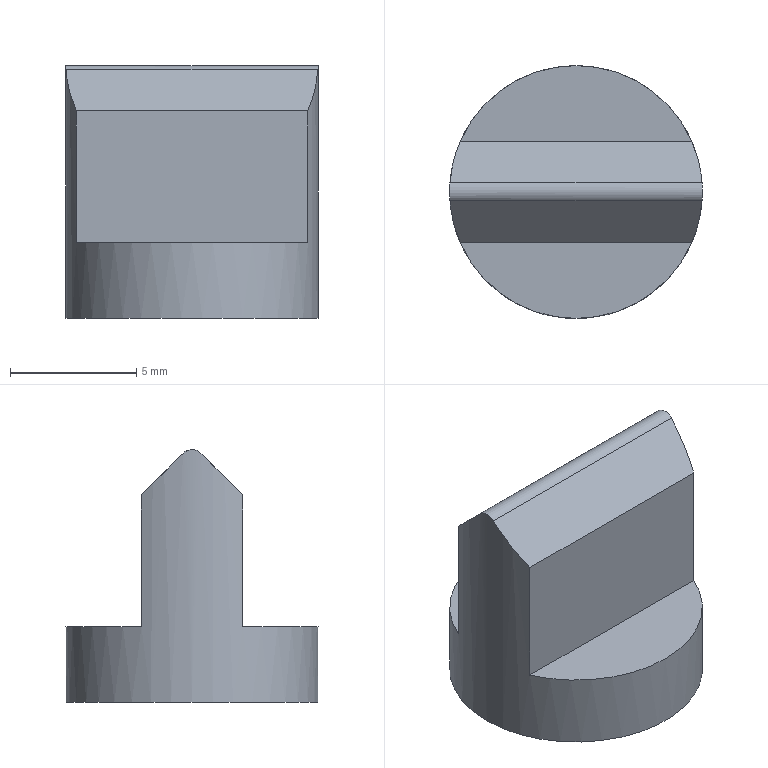Part | STEP file | lll_id294_x_t | 1 solid | 9 faces | box 10 x 10 x 10 mm | volume 477.247 mm3 | plane 7 | cylinder 2 | commonest cylinder face diameters 1 x1 10 x1
STEP:
#1=CARTESIAN_POINT('',(5.,106.,-20.));
#2=VERTEX_POINT('',#1);
#3=CARTESIAN_POINT('',(0.,106.,-20.));
#4=DIRECTION('',(0.,0.,1.));
#5=DIRECTION('',(1.,0.,0.));
#6=AXIS2_PLACEMENT_3D('',#3,#4,#5);
#7=CIRCLE('',#6,5.);
#8=EDGE_CURVE('',#2,#2,#7,.T.);
#9=ORIENTED_EDGE('',*,*,#8,.F.);
#10=EDGE_LOOP('',(#9));
#11=FACE_OUTER_BOUND('',#10,.T.);
#12=CARTESIAN_POINT('',(48.194,357.,-20.));
#13=DIRECTION('',(0.,0.,-1.));
#14=DIRECTION('',(1.,0.,0.));
#15=AXIS2_PLACEMENT_3D('',#12,#13,#14);
#16=PLANE('',#15);
#17=ADVANCED_FACE('',(#11),#16,.T.);
#18=CARTESIAN_POINT('',(-4.583,104.,-17.));
#19=VERTEX_POINT('',#18);
#20=CARTESIAN_POINT('',(-4.583,104.,-11.793));
#21=VERTEX_POINT('',#20);
#22=CARTESIAN_POINT('',(-4.583,104.,-22.));
#23=DIRECTION('',(0.,0.,1.));
#24=VECTOR('',#23,1.);
#25=LINE('',#22,#24);
#26=EDGE_CURVE('',#19,#21,#25,.T.);
#27=ORIENTED_EDGE('',*,*,#26,.F.);
#28=CARTESIAN_POINT('',(4.583,104.,-17.));
#29=VERTEX_POINT('',#28);
#30=CARTESIAN_POINT('',(13.,104.,-17.));
#31=DIRECTION('',(-1.,0.,0.));
#32=VECTOR('',#31,1.);
#33=LINE('',#30,#32);
#34=EDGE_CURVE('',#29,#19,#33,.T.);
#35=ORIENTED_EDGE('',*,*,#34,.F.);
#36=CARTESIAN_POINT('',(4.583,104.,-11.793));
#37=VERTEX_POINT('',#36);
#38=CARTESIAN_POINT('',(4.583,104.,-22.));
#39=DIRECTION('',(0.,0.,-1.));
#40=VECTOR('',#39,1.);
#41=LINE('',#38,#40);
#42=EDGE_CURVE('',#37,#29,#41,.T.);
#43=ORIENTED_EDGE('',*,*,#42,.F.);
#44=CARTESIAN_POINT('',(13.,104.,-11.793));
#45=DIRECTION('',(-1.,0.,0.));
#46=VECTOR('',#45,1.);
#47=LINE('',#44,#46);
#48=EDGE_CURVE('',#37,#21,#47,.T.);
#49=ORIENTED_EDGE('',*,*,#48,.T.);
#50=EDGE_LOOP('',(#27,#35,#43,#49));
#51=FACE_OUTER_BOUND('',#50,.T.);
#52=CARTESIAN_POINT('',(13.,104.,-11.5));
#53=DIRECTION('',(0.,1.,0.));
#54=DIRECTION('',(0.,0.,-1.));
#55=AXIS2_PLACEMENT_3D('',#52,#53,#54);
#56=PLANE('',#55);
#57=ADVANCED_FACE('',(#51),#56,.F.);
#58=CARTESIAN_POINT('',(-4.583,108.,-17.));
#59=VERTEX_POINT('',#58);
#60=CARTESIAN_POINT('',(4.583,108.,-17.));
#61=VERTEX_POINT('',#60);
#62=CARTESIAN_POINT('',(0.,106.,-17.));
#63=DIRECTION('',(0.,0.,-1.));
#64=DIRECTION('',(1.,0.,0.));
#65=AXIS2_PLACEMENT_3D('',#62,#63,#64);
#66=CIRCLE('',#65,5.);
#67=EDGE_CURVE('',#59,#61,#66,.T.);
#68=ORIENTED_EDGE('',*,*,#67,.F.);
#69=CARTESIAN_POINT('',(13.,108.,-17.));
#70=DIRECTION('',(-1.,0.,0.));
#71=VECTOR('',#70,1.);
#72=LINE('',#69,#71);
#73=EDGE_CURVE('',#61,#59,#72,.T.);
#74=ORIENTED_EDGE('',*,*,#73,.F.);
#75=EDGE_LOOP('',(#68,#74));
#76=FACE_OUTER_BOUND('',#75,.T.);
#77=CARTESIAN_POINT('',(13.,111.,-17.));
#78=DIRECTION('',(0.,0.,-1.));
#79=DIRECTION('',(0.,-1.,0.));
#80=AXIS2_PLACEMENT_3D('',#77,#78,#79);
#81=PLANE('',#80);
#82=ADVANCED_FACE('',(#76),#81,.F.);
#83=CARTESIAN_POINT('',(4.583,108.,-11.793));
#84=VERTEX_POINT('',#83);
#85=CARTESIAN_POINT('',(4.583,108.,-22.));
#86=DIRECTION('',(0.,0.,1.));
#87=VECTOR('',#86,1.);
#88=LINE('',#85,#87);
#89=EDGE_CURVE('',#61,#84,#88,.T.);
#90=ORIENTED_EDGE('',*,*,#89,.F.);
#91=ORIENTED_EDGE('',*,*,#73,.T.);
#92=CARTESIAN_POINT('',(-4.583,108.,-11.793));
#93=VERTEX_POINT('',#92);
#94=CARTESIAN_POINT('',(-4.583,108.,-22.));
#95=DIRECTION('',(0.,0.,-1.));
#96=VECTOR('',#95,1.);
#97=LINE('',#94,#96);
#98=EDGE_CURVE('',#93,#59,#97,.T.);
#99=ORIENTED_EDGE('',*,*,#98,.F.);
#100=CARTESIAN_POINT('',(13.,108.,-11.793));
#101=DIRECTION('',(-1.,0.,0.));
#102=VECTOR('',#101,1.);
#103=LINE('',#100,#102);
#104=EDGE_CURVE('',#84,#93,#103,.T.);
#105=ORIENTED_EDGE('',*,*,#104,.F.);
#106=EDGE_LOOP('',(#90,#91,#99,#105));
#107=FACE_OUTER_BOUND('',#106,.T.);
#108=CARTESIAN_POINT('',(13.,108.,-17.));
#109=DIRECTION('',(0.,-1.,0.));
#110=DIRECTION('',(0.,0.,1.));
#111=AXIS2_PLACEMENT_3D('',#108,#109,#110);
#112=PLANE('',#111);
#113=ADVANCED_FACE('',(#107),#112,.F.);
#114=CARTESIAN_POINT('',(-4.987,106.354,-10.146));
#115=VERTEX_POINT('',#114);
#116=CARTESIAN_POINT('',(0.,106.,-9.793));
#117=DIRECTION('',(0.,-0.7071,-0.7071));
#118=DIRECTION('',(0.,-0.7071,0.7071));
#119=AXIS2_PLACEMENT_3D('',#116,#117,#118);
#120=ELLIPSE('',#119,7.071,5.);
#121=EDGE_CURVE('',#115,#93,#120,.T.);
#122=ORIENTED_EDGE('',*,*,#121,.F.);
#123=CARTESIAN_POINT('',(4.987,106.354,-10.146));
#124=VERTEX_POINT('',#123);
#125=CARTESIAN_POINT('',(13.,106.354,-10.146));
#126=DIRECTION('',(-1.,0.,0.));
#127=VECTOR('',#126,1.);
#128=LINE('',#125,#127);
#129=EDGE_CURVE('',#124,#115,#128,.T.);
#130=ORIENTED_EDGE('',*,*,#129,.F.);
#131=CARTESIAN_POINT('',(0.,106.,-9.793));
#132=DIRECTION('',(0.,-0.7071,-0.7071));
#133=DIRECTION('',(0.,-0.7071,0.7071));
#134=AXIS2_PLACEMENT_3D('',#131,#132,#133);
#135=ELLIPSE('',#134,7.071,5.);
#136=EDGE_CURVE('',#84,#124,#135,.T.);
#137=ORIENTED_EDGE('',*,*,#136,.F.);
#138=ORIENTED_EDGE('',*,*,#104,.T.);
#139=EDGE_LOOP('',(#122,#130,#137,#138));
#140=FACE_OUTER_BOUND('',#139,.T.);
#141=CARTESIAN_POINT('',(13.,107.707,-11.5));
#142=DIRECTION('',(0.,-0.7071,-0.7071));
#143=DIRECTION('',(0.,-0.7071,0.7071));
#144=AXIS2_PLACEMENT_3D('',#141,#142,#143);
#145=PLANE('',#144);
#146=ADVANCED_FACE('',(#140),#145,.F.);
#147=CARTESIAN_POINT('',(4.987,105.646,-10.146));
#148=VERTEX_POINT('',#147);
#149=CARTESIAN_POINT('',(4.987,106.354,-10.146));
#150=CARTESIAN_POINT('',(4.99,106.317,-10.11));
#151=CARTESIAN_POINT('',(4.993,106.275,-10.079));
#152=CARTESIAN_POINT('',(4.995,106.229,-10.056));
#153=CARTESIAN_POINT('',(4.997,106.18,-10.03));
#154=CARTESIAN_POINT('',(4.999,106.124,-10.012));
#155=CARTESIAN_POINT('',(5.,106.069,-10.005));
#156=CARTESIAN_POINT('',(5.,106.014,-9.997));
#157=CARTESIAN_POINT('',(5.,105.956,-9.999));
#158=CARTESIAN_POINT('',(4.999,105.902,-10.01));
#159=CARTESIAN_POINT('',(4.998,105.847,-10.021));
#160=CARTESIAN_POINT('',(4.996,105.794,-10.041));
#161=CARTESIAN_POINT('',(4.994,105.746,-10.07));
#162=CARTESIAN_POINT('',(4.992,105.71,-10.091));
#163=CARTESIAN_POINT('',(4.99,105.676,-10.117));
#164=CARTESIAN_POINT('',(4.987,105.646,-10.146));
#165=B_SPLINE_CURVE_WITH_KNOTS('',3,(#149,#150,#151,#152,#153,#154,#155,#156,#157,#158,#159,#160,#161,#162,#163,#164),.UNSPECIFIED.,.F.,.F.,(4,3,3,3,3,4),(0.,0.1968,0.4121,0.6258,0.8395,1.),.UNSPECIFIED.);
#166=EDGE_CURVE('',#124,#148,#165,.T.);
#167=ORIENTED_EDGE('',*,*,#166,.F.);
#168=ORIENTED_EDGE('',*,*,#129,.T.);
#169=CARTESIAN_POINT('',(-4.987,105.646,-10.146));
#170=VERTEX_POINT('',#169);
#171=CARTESIAN_POINT('',(-4.987,105.646,-10.146));
#172=CARTESIAN_POINT('',(-4.99,105.683,-10.11));
#173=CARTESIAN_POINT('',(-4.993,105.725,-10.079));
#174=CARTESIAN_POINT('',(-4.995,105.771,-10.056));
#175=CARTESIAN_POINT('',(-4.997,105.82,-10.03));
#176=CARTESIAN_POINT('',(-4.999,105.876,-10.012));
#177=CARTESIAN_POINT('',(-5.,105.931,-10.005));
#178=CARTESIAN_POINT('',(-5.,105.986,-9.997));
#179=CARTESIAN_POINT('',(-5.,106.044,-9.999));
#180=CARTESIAN_POINT('',(-4.999,106.098,-10.01));
#181=CARTESIAN_POINT('',(-4.998,106.153,-10.021));
#182=CARTESIAN_POINT('',(-4.996,106.206,-10.041));
#183=CARTESIAN_POINT('',(-4.994,106.254,-10.07));
#184=CARTESIAN_POINT('',(-4.992,106.29,-10.091));
#185=CARTESIAN_POINT('',(-4.99,106.324,-10.117));
#186=CARTESIAN_POINT('',(-4.987,106.354,-10.146));
#187=B_SPLINE_CURVE_WITH_KNOTS('',3,(#171,#172,#173,#174,#175,#176,#177,#178,#179,#180,#181,#182,#183,#184,#185,#186),.UNSPECIFIED.,.F.,.F.,(4,3,3,3,3,4),(0.,0.1968,0.4121,0.6258,0.8395,1.),.UNSPECIFIED.);
#188=EDGE_CURVE('',#170,#115,#187,.T.);
#189=ORIENTED_EDGE('',*,*,#188,.F.);
#190=CARTESIAN_POINT('',(13.,105.646,-10.146));
#191=DIRECTION('',(-1.,0.,0.));
#192=VECTOR('',#191,1.);
#193=LINE('',#190,#192);
#194=EDGE_CURVE('',#148,#170,#193,.T.);
#195=ORIENTED_EDGE('',*,*,#194,.F.);
#196=EDGE_LOOP('',(#167,#168,#189,#195));
#197=FACE_OUTER_BOUND('',#196,.T.);
#198=CARTESIAN_POINT('',(13.,106.,-10.5));
#199=DIRECTION('',(-1.,0.,0.));
#200=DIRECTION('',(0.,0.,1.));
#201=AXIS2_PLACEMENT_3D('',#198,#199,#200);
#202=CYLINDRICAL_SURFACE('',#201,0.5);
#203=ADVANCED_FACE('',(#197),#202,.T.);
#204=CARTESIAN_POINT('',(0.,106.,-9.793));
#205=DIRECTION('',(0.,0.7071,-0.7071));
#206=DIRECTION('',(0.,0.7071,0.7071));
#207=AXIS2_PLACEMENT_3D('',#204,#205,#206);
#208=ELLIPSE('',#207,7.071,5.);
#209=EDGE_CURVE('',#148,#37,#208,.T.);
#210=ORIENTED_EDGE('',*,*,#209,.F.);
#211=ORIENTED_EDGE('',*,*,#194,.T.);
#212=CARTESIAN_POINT('',(0.,106.,-9.793));
#213=DIRECTION('',(0.,0.7071,-0.7071));
#214=DIRECTION('',(0.,0.7071,0.7071));
#215=AXIS2_PLACEMENT_3D('',#212,#213,#214);
#216=ELLIPSE('',#215,7.071,5.);
#217=EDGE_CURVE('',#21,#170,#216,.T.);
#218=ORIENTED_EDGE('',*,*,#217,.F.);
#219=ORIENTED_EDGE('',*,*,#48,.F.);
#220=EDGE_LOOP('',(#210,#211,#218,#219));
#221=FACE_OUTER_BOUND('',#220,.T.);
#222=CARTESIAN_POINT('',(13.,105.646,-10.146));
#223=DIRECTION('',(0.,0.7071,-0.7071));
#224=DIRECTION('',(0.,-0.7071,-0.7071));
#225=AXIS2_PLACEMENT_3D('',#222,#223,#224);
#226=PLANE('',#225);
#227=ADVANCED_FACE('',(#221),#226,.F.);
#228=CARTESIAN_POINT('',(0.,106.,-17.));
#229=DIRECTION('',(0.,0.,-1.));
#230=DIRECTION('',(1.,0.,0.));
#231=AXIS2_PLACEMENT_3D('',#228,#229,#230);
#232=CIRCLE('',#231,5.);
#233=EDGE_CURVE('',#29,#19,#232,.T.);
#234=ORIENTED_EDGE('',*,*,#233,.F.);
#235=ORIENTED_EDGE('',*,*,#34,.T.);
#236=EDGE_LOOP('',(#234,#235));
#237=FACE_OUTER_BOUND('',#236,.T.);
#238=CARTESIAN_POINT('',(13.,104.,-17.));
#239=DIRECTION('',(0.,0.,-1.));
#240=DIRECTION('',(0.,-1.,0.));
#241=AXIS2_PLACEMENT_3D('',#238,#239,#240);
#242=PLANE('',#241);
#243=ADVANCED_FACE('',(#237),#242,.F.);
#244=ORIENTED_EDGE('',*,*,#8,.T.);
#245=EDGE_LOOP('',(#244));
#246=FACE_BOUND('',#245,.T.);
#247=ORIENTED_EDGE('',*,*,#98,.T.);
#248=ORIENTED_EDGE('',*,*,#67,.T.);
#249=ORIENTED_EDGE('',*,*,#89,.T.);
#250=ORIENTED_EDGE('',*,*,#136,.T.);
#251=ORIENTED_EDGE('',*,*,#166,.T.);
#252=ORIENTED_EDGE('',*,*,#209,.T.);
#253=ORIENTED_EDGE('',*,*,#42,.T.);
#254=ORIENTED_EDGE('',*,*,#233,.T.);
#255=ORIENTED_EDGE('',*,*,#26,.T.);
#256=ORIENTED_EDGE('',*,*,#217,.T.);
#257=ORIENTED_EDGE('',*,*,#188,.T.);
#258=ORIENTED_EDGE('',*,*,#121,.T.);
#259=EDGE_LOOP('',(#247,#248,#249,#250,#251,#252,#253,#254,#255,#256,#257,#258));
#260=FACE_BOUND('',#259,.T.);
#261=CARTESIAN_POINT('',(0.,106.,-22.));
#262=DIRECTION('',(0.,0.,1.));
#263=DIRECTION('',(1.,0.,0.));
#264=AXIS2_PLACEMENT_3D('',#261,#262,#263);
#265=CYLINDRICAL_SURFACE('',#264,5.);
#266=ADVANCED_FACE('',(#246,#260),#265,.T.);
#267=CLOSED_SHELL('',(#17,#57,#82,#113,#146,#203,#227,#243,#266));
#268=MANIFOLD_SOLID_BREP('',#267);
#269=(LENGTH_UNIT()NAMED_UNIT(*)SI_UNIT(.MILLI.,.METRE.));
#270=UNCERTAINTY_MEASURE_WITH_UNIT(LENGTH_MEASURE(0.0508),#269,'','');
#271=(NAMED_UNIT(*)PLANE_ANGLE_UNIT()SI_UNIT($,.RADIAN.));
#272=PLANE_ANGLE_MEASURE_WITH_UNIT(PLANE_ANGLE_MEASURE(0.01745),#271);
#273=DIMENSIONAL_EXPONENTS(0.,0.,0.,0.,0.,0.,0.);
#274=(CONVERSION_BASED_UNIT('DEGREE',#272)NAMED_UNIT(#273)PLANE_ANGLE_UNIT());
#275=(NAMED_UNIT(*)SI_UNIT($,.STERADIAN.)SOLID_ANGLE_UNIT());
#276=(GEOMETRIC_REPRESENTATION_CONTEXT(3)GLOBAL_UNCERTAINTY_ASSIGNED_CONTEXT((#270))GLOBAL_UNIT_ASSIGNED_CONTEXT((#269,#274,#275))REPRESENTATION_CONTEXT('',''));
#277=ADVANCED_BREP_SHAPE_REPRESENTATION('',(#268),#276);